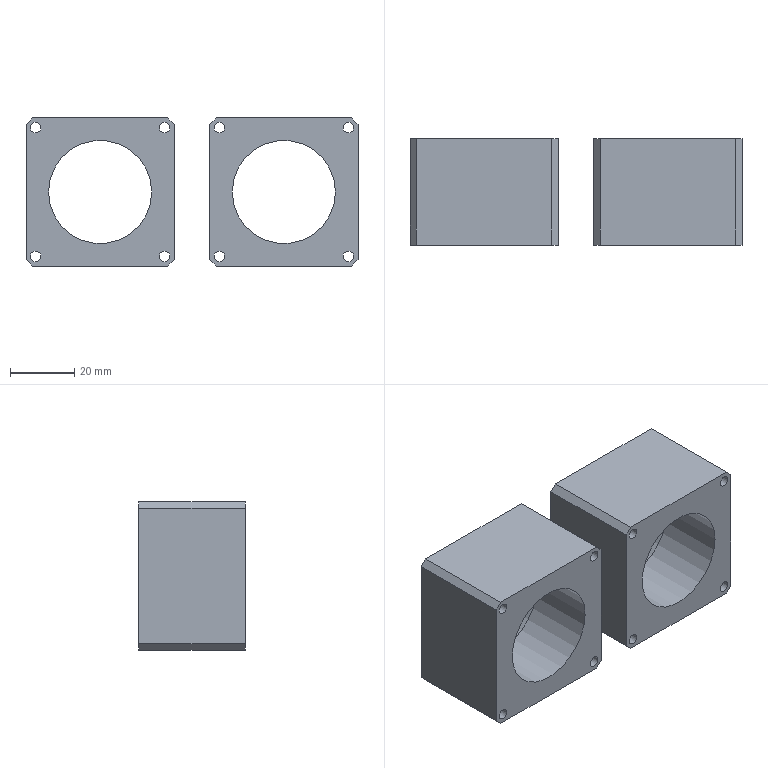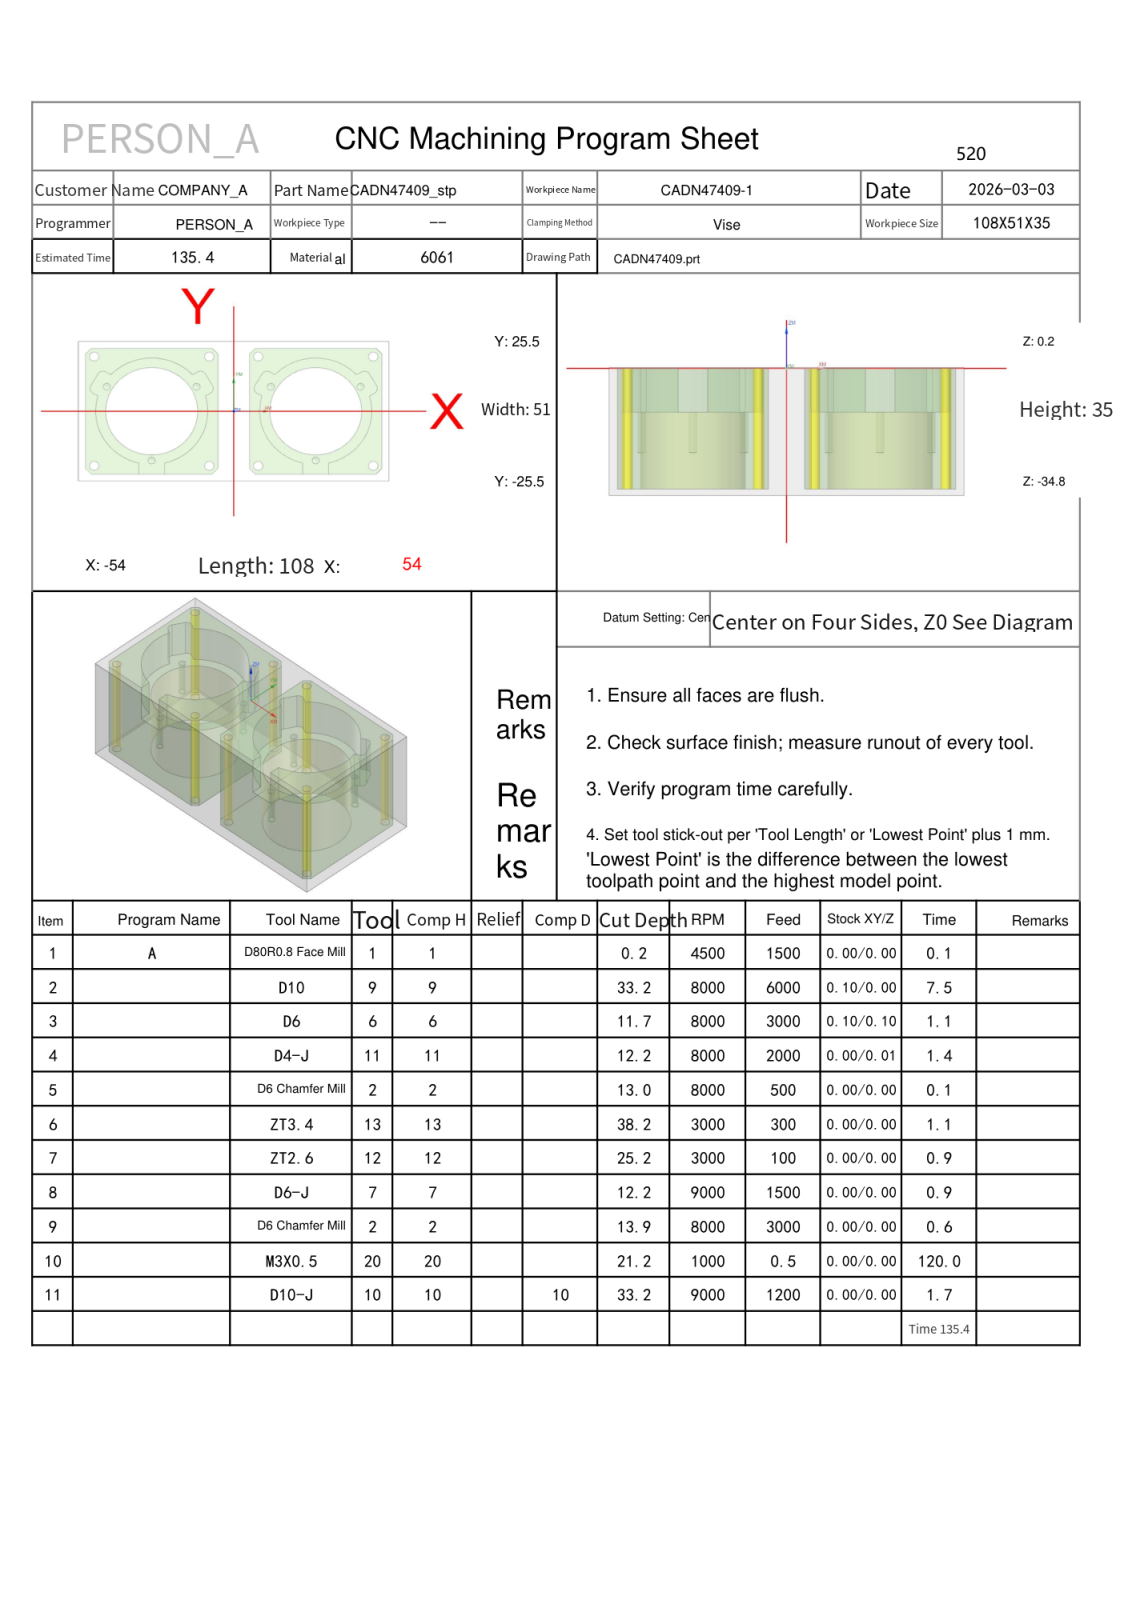NC program | NX | posted by the shop | part box 103 x 33 x 46 mm
Lines 1 to 36 of 11287:
%
O0001
(Machine time: 245.21 MIN)
(===Total Tool:10===)
(T1=D80R0.8 Face Mill  D=80.  R=0.8  D-  H01 Z=0.    )
(T9=D10     D=10.  R=0.   D-  H09 Z=-33.  )
(T6=D6      D=6.   R=0.   D-  H06 Z=-11.5 )
(T11=D4-J   D=4.   R=0.   D-  H11 Z=-12.  )
(T2=D6 Chamfer Mill    D=6.   R=0.   D-  H02 Z=-13.75)
(T13=ZT3.4  D=3.4  DR_a=118 D-  H13 Z=-38.  )
(T12=ZT2.6  D=2.6  DR_a=118 D-  H12 Z=-25.  )
(T7=D6-J    D=6.   R=0.   D7  H07 Z=-12.  )
(T20=M3X0.5 D=2.5  DR_a=180 D-  H20 Z=-21.  )
(T10=D10-J  D=10.  R=0.   D10 H10 Z=-33.  )
G80 G90 G17 G49 G40
G91 G28 Z0
M01
N1 T01 M06
(D80R0.8 Face Mill   D=80. R=0.8 H=01 ce=0.00 di=0.00)
G00 G90 G54 X-96.5 Y0.0 M03 S4500
G43 H01 Z50.
M08
Z2.
G01 Z0.0 F1500.
X-91.5
X91.5
X96.5
Z2.
G00 Z50.
G91 G28 Z0.0
M05
M09
G91 G28 Z0.0
M01